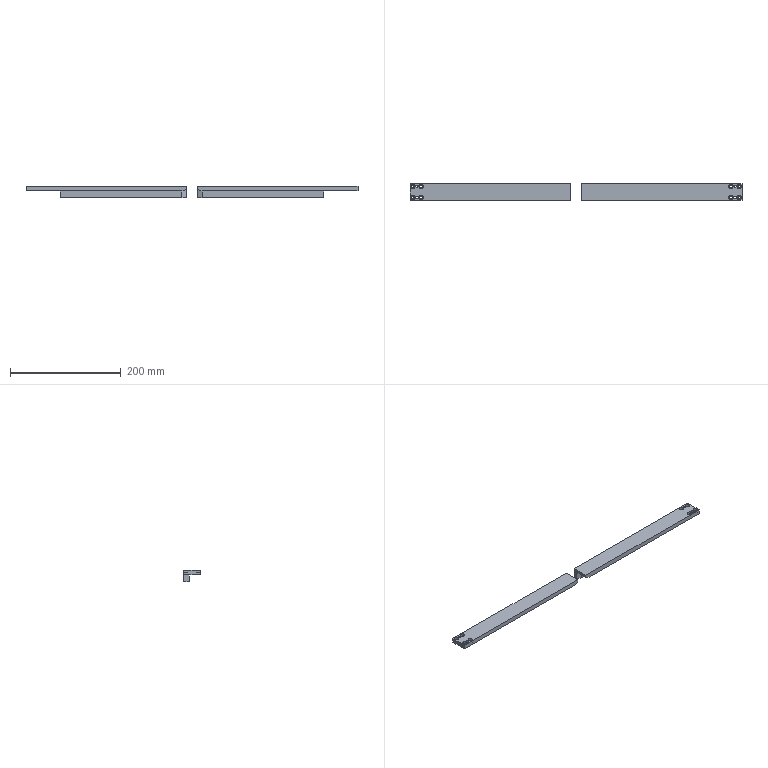NC program | NX | posted with a generic post | part box 600 x 30 x 20 mm
Whole program:
N10 G17 G21 G94 G90
(FLOOR_WALL_COPY_1 , TOOL : D50)
N12 T01 M6
N14 G54
N16 G17 G0 G90 X173. Y0. S6500 M3
N18 G43 Z30. H1
N20 Z7.
N22 G94 G1 Z4. F1250.
N24 X170.
N26 X-170.
N28 X-173.
N30 Z7.
N32 G0 Z30.
N34 X173.
N36 Z6.
N38 G1 Z3.
N40 X170.
N42 X-170.
N44 X-173.
N46 Z6.
N48 G0 Z30.
N50 X173.
N52 Z5.
N54 G1 Z2.
N56 X170.
N58 X-170.
N60 X-173.
N62 Z5.
N64 G0 Z30.
N66 X173.
N68 Z4.
N70 G1 Z1.
N72 X170.
N74 X-170.
N76 X-173.
N78 Z4.
N80 G0 Z30.
N82 X173.
N84 Z3.
N86 G1 Z0.
N88 X170.
N90 X-170.
N92 X-173.
N94 Z3.
N96 G0 Z30.
N98 M5
(FLOOR_WALL_1_1 , TOOL : D10)
N100 T03 M6
N102 G54
N104 G17 G0 G90 X-148.459 Y-23.147 S7000 M3
N106 G43 Z30. H3
N108 Z-8.85
N110 G94 G1 Z-11.85 F1000.
N112 X-149.446 Y-20.147
N114 G2 X-150.147 Y-17.873 R64. F3000.
N116 G1 Y-13.829
N118 G3 X-148.392 Y-20.147 R63.
N120 G1 X-147.337
N122 G2 X-150.147 Y-8.032 R62.
N124 G1 X-150.528 Y-5.056
N126 X-153.147
N128 Z-8.85
N130 G0 Z30.
N132 X-149.65 Y23.147
N134 Z-8.85
N136 G1 Z-11.85 F1000.
N138 Y20.147
N140 Y-0.15 F3000.
N142 G3 X-146.279 Y-20.147 R61.
N144 G1 X-145.22
N146 G2 X-148.65 Y-0.15 R60.
N148 G1 Y20.147
N150 X-147.65
N152 Y-0.15
N154 G3 X-144.158 Y-20.147 R59.
N156 G1 X-143.094
N158 G2 X-146.65 Y-0.15 R58.
N160 G1 Y20.147
N162 X-145.65
N164 Y-0.15
N166 G3 X-142.027 Y-20.147 R57.
N168 G1 X-140.958
N170 G2 X-144.65 Y-0.15 R56.
N172 G1 Y20.147
N174 X-143.65
N176 Y-0.15
N178 G3 X-139.886 Y-20.147 R55.
N180 G1 X-138.811
N182 G2 X-142.65 Y-0.15 R54.
N184 G1 Y20.147
N186 X-141.65
N188 Y-0.15
N190 G3 X-137.733 Y-20.147 R53.
N192 G1 X-136.651
N194 G2 X-140.65 Y-0.15 R52.
N196 G1 Y20.147
N198 X-139.65
N200 Y-0.15
N202 G3 X-135.566 Y-20.147 R51.
N204 G1 X-134.477
N206 G2 X-138.65 Y-0.15 R50.
N208 G1 Y20.147
N210 X-137.65
N212 Y-0.15
N214 G3 X-133.384 Y-20.147 R49.
N216 G1 X-132.286
N218 G2 X-136.65 Y-0.15 R48.
N220 G1 Y20.147
N222 X-135.65
N224 Y-0.15
N226 G3 X-131.184 Y-20.147 R47.
N228 G1 X-130.076
N230 G2 X-134.65 Y-0.15 R46.
N232 G1 Y20.147
N234 X-133.65
N236 Y-0.15
N238 G3 X-128.963 Y-20.147 R45.
N240 G1 X-127.843
N242 G2 X-132.65 Y-0.15 R44.
N244 G1 Y20.147
N246 X-131.65
N248 Y-0.15
N250 G3 X-126.717 Y-20.147 R43.
N252 G1 X-125.584
N254 G2 X-130.65 Y-0.15 R42.
N256 G1 Y20.147
N258 X-129.65
N260 Y-0.15
N262 G3 X-124.443 Y-20.147 R41.
N264 G1 X-123.293
N266 G2 X-128.65 Y-0.15 R40.
N268 G1 Y20.147
N270 X-127.65
N272 Y-0.15
N274 G3 X-122.133 Y-20.147 R39.
N276 G1 X-120.963
N278 G2 X-126.65 Y-0.15 R38.
N280 G1 Y20.147
N282 X-125.65
N284 Y-0.15
N286 G3 X-119.781 Y-20.147 R37.
N288 G1 X-118.585
N290 G2 X-124.65 Y-0.15 R36.
N292 G1 Y20.147
N294 X-123.65
N296 Y-0.15
N298 G3 X-117.375 Y-20.147 R35.
N300 G1 X-116.148
N302 G2 X-122.65 Y-0.15 R34.
N304 G1 Y20.147
N306 X-121.65
N308 Y-0.15
N310 G3 X-114.901 Y-20.147 R33.
N312 G1 X-113.632
N314 G2 X-120.65 Y-0.15 R32.
N316 G1 Y20.147
N318 X-119.65
N320 Y-0.15
N322 G3 X-112.338 Y-20.147 R31.
N324 G1 X-111.013
N326 G2 X-118.65 Y-0.15 R30.
N328 G1 Y20.147
N330 X-117.65
N332 Y-0.15
N334 G3 X-109.653 Y-20.147 R29.
N336 G1 X-108.249
N338 G2 X-116.65 Y-0.15 R28.
N340 G1 Y20.147
N342 X-115.65
N344 Y-0.15
N346 G3 X-106.792 Y-20.147 R27.
N348 G1 X-105.267
N350 G2 X-114.65 Y-0.15 R26.
N352 G1 Y20.147
N354 X-113.65
N356 Y-0.15
N358 G3 X-103.654 Y-20.147 R25.
N360 G1 X-101.921
N362 G2 X-112.65 Y-0.15 R24.
N364 G1 Y20.147
N366 X-111.65
N368 Y-0.15
N370 G3 X-100.013 Y-20.147 R23.
N372 G1 X-97.822
N374 G2 X-110.65 Y-0.15 R22.
N376 G1 Y20.147
N378 X-109.65
N380 Y-0.15
N382 G3 X-95.062 Y-20.147 R21.
N384 G1 X-88.996
N386 G2 X-108.65 Y-0.15 R20.
N388 G1 Y20.147
N390 Y23.147
N392 Z-8.85
N394 G0 Z30.
N396 X141.729 Y-23.147
N398 Z-8.85
N400 G1 Z-11.85 F1000.
N402 X149.972 Y-20.147
N404 X150.147 Y-20.083 F3000.
N406 Y-19.019
N408 X147.048 Y-20.147
N410 X144.078
N412 G3 X144.848 Y-19.884 R21.
N414 G1 X150.147 Y-17.955
N416 Y-16.891
N418 X144.506 Y-18.944
N420 G2 X138.012 Y-20.147 R20.
N422 G1 X135.012 Y-20.199
N424 Y-23.147
N426 Z-8.85
N428 G0 Z30.
N430 X-107.65 Y23.147
N432 Z-8.85
N434 G1 Z-11.85 F1000.
N436 Y20.147
N438 Y-0.15 F3000.
N440 G3 X-88.65 Y-19.15 R19.
N442 G1 X137.666
N444 G3 X144.164 Y-18.004 R19.
N446 G1 X150.147 Y-15.827
N448 Y-15.
N450 Y-14.762
N452 X143.822 Y-17.064
N454 G2 X137.666 Y-18.15 R18.
N456 G1 X-88.65
N458 G2 X-106.65 Y-0.15 R18.
N460 G1 Y20.147
N462 X-105.65
N464 Y-0.15
N466 G3 X-88.65 Y-17.15 R17.
N468 G1 X137.666
N470 G3 X143.48 Y-16.125 R17.
N472 G1 X150.147 Y-13.698
N474 Y-12.634
N476 X143.138 Y-15.185
N478 G2 X137.666 Y-16.15 R16.
N480 G1 X-88.65
N482 G2 X-104.65 Y-0.15 R16.
N484 G1 Y20.147
N486 X-103.65
N488 Y-0.15
N490 G3 X-88.65 Y-15.15 R15.
N492 G1 X137.666
N494 G3 X142.796 Y-14.245 R15.
N496 G1 X150.147 Y-11.57
N498 Y-10.506
N500 X142.454 Y-13.306
N502 G2 X137.666 Y-14.15 R14.
N504 G1 X-88.65
N506 G2 X-102.65 Y-0.15 R14.
N508 G1 Y20.147
N510 X-101.65
N512 Y-0.15
N514 G3 X-88.65 Y-13.15 R13.
N516 G1 X137.666
N518 G3 X142.112 Y-12.366 R13.
N520 G1 X150.147 Y-9.441
N522 Y-8.377
N524 X141.77 Y-11.426
N526 G2 X137.666 Y-12.15 R12.
N528 G1 X-88.65
N530 G2 X-100.65 Y-0.15 R12.
N532 G1 Y20.147
N534 X-99.65
N536 Y-0.15
N538 G3 X-88.65 Y-11.15 R11.
N540 G1 X137.666
N542 G3 X141.428 Y-10.487 R11.
N544 G1 X150.147 Y-7.313
N546 Y-6.249
N548 X141.086 Y-9.547
N550 G2 X137.666 Y-10.15 R10.
N552 G1 X-88.65
N554 G2 X-98.65 Y-0.15 R10.
N556 G1 Y20.147
N558 X-97.65
N560 Y-0.15
N562 G3 X-88.65 Y-9.15 R9.
N564 G1 X137.666
N566 G3 X140.744 Y-8.607 R9.
N568 G1 X150.147 Y-5.185
N570 Y-4.121
N572 X140.402 Y-7.668
N574 G2 X137.666 Y-8.15 R8.
N576 G1 X-88.65
N578 G2 X-96.65 Y-0.15 R8.
N580 G1 Y20.147
N582 X-95.65
N584 Y-0.15
N586 G3 X-88.65 Y-7.15 R7.
N588 G1 X137.666
N590 G3 X140.06 Y-6.728 R7.
N592 G1 X150.147 Y-3.056
N594 Y-1.992
N596 X139.718 Y-5.788
N598 G2 X137.666 Y-6.15 R6.
N600 G1 X-88.65
N602 G2 X-94.65 Y-0.15 R6.
N604 G1 Y20.147
N606 X-93.65
N608 Y-0.15
N610 G3 X-88.65 Y-5.15 R5.
N612 G1 X137.666
N614 G3 X139.376 Y-4.848 R5.
N616 G1 X150.147 Y-0.928
N618 Y0.136
N620 X139.034 Y-3.909
N622 G2 X137.666 Y-4.15 R4.
N624 G1 X-88.65
N626 G2 X-92.65 Y-0.15 R4.
N628 G1 Y20.147
N630 X-91.65
N632 Y-0.15
N634 G3 X-88.65 Y-3.15 R3.
N636 G1 X137.666
N638 G3 X138.692 Y-2.969 R3.
N640 G1 X150.147 Y1.2
N642 Y2.264
N644 X138.35 Y-2.029
N646 G2 X137.666 Y-2.15 R2.
N648 G1 X-88.65
N650 G2 X-90.65 Y-0.15 R2.
N652 G1 Y20.147
N654 X-89.65
N656 Y-0.15
N658 G3 X-88.65 Y-1.15 R1.
N660 G1 X137.666
N662 G3 X138.008 Y-1.09 R1.
N664 G1 X150.147 Y3.329
N666 Y4.393
N668 X137.666 Y-0.15
N670 X-88.65
N672 Y20.147
N674 Y23.15
N676 Z-8.85
N678 G0 Z30.
N680 M5
(FLOOR_WALL_1_COPY_1_1 , TOOL : D10JING)
N682 T04 M6
N684 G54
N686 G17 G0 G90 X151.139 Y-20.974 S7000 M3
N688 G43 Z30. H4
N690 Z-10.5
N692 G94 G1 Z-12. F1000.
N694 X150.865 Y-20.499
N696 G3 X149.999 Y-19.999 R1.
N698 G1 X-149.999
N700 Y-15.571
N702 X149.999
N704 Y-11.142
N706 X-149.999
N708 Y-6.714
N710 X149.999
N712 Y-2.286
N714 X-149.999
N716 Y2.142
N718 X-89.
N720 Y6.571
N722 X-149.999
N724 Y10.999
N726 X-89.
N728 Y15.427
N730 X-149.999
N732 G3 X-150.865 Y14.927 R1.
N734 G1 X-151.499 Y13.829
N736 Z-10.5
N738 G0 Z-8.9
N740 G1 X-89. Y2.142 F6000.
N742 G0 Z-10.5
N744 G1 Z-12. F1000.
N746 Y0.
N748 G3 X-88.5 Y-0.5 R0.5
N750 G1 X137.639
N752 X137.728 Y-0.502
N754 X137.81 Y-0.47
N756 X144.987 Y2.142
N758 X149.999
N760 G2 X150.865 Y1.642 R1.
N762 G1 X151.499 Y0.544
N764 Z-10.5
N766 G0 Z-8.9
N768 G1 X151.5 Y3.892 F6000.
N770 G0 Z-10.5
N772 G1 Z-12. F1000.
N774 X150.984 Y4.325
N776 G3 X149.999 Y4.499 R1.
N778 G1 X137.639 Y0.
N780 X-88.5
N782 Y19.999
N784 G3 X-89. Y20.865 R1.
N786 G1 X-90.098 Y21.499
N788 Z-10.5
N790 G0 Z30.
N792 M5
(ZLEVEL_PROFILE_COPY_COPY_1_COPY_COPY_COPY_1_COPY_COPY_1 , TOOL : D6R0.5)
N794 T20 M6
N796 G54
N798 G17 G0 G90 X139.958 Y-16.121 S7000 M3
N800 G43 Z30. H20
N802 Z-12.034
N804 G94 G1 X139.738 Y-15.994 F1000.
N806 G2 X139.439 Y-15.474 R0.6
N808 G1 X139.44 Y-15. F3000.
N810 Y2.784
N812 X139.534 Y2.818 Z-12.068
N814 Y-15.
N816 X139.533 Y-15.474
N818 X139.581 Y-15.475 Z-12.086
N820 X139.627 Z-12.103
N822 X139.628 Y-15.
N824 Y2.852
N826 X139.722 Y2.886 Z-12.137
N828 Y-15.
N830 X139.721 Y-15.476
N832 X139.769 Z-12.154
N834 X139.815 Z-12.171
N836 X139.816 Y-15.
N838 Y2.92
N840 X139.91 Y2.955 Z-12.205
N842 Y-15.
N844 X139.909 Y-15.477
N846 X139.957 Z-12.222
N848 X140.003 Z-12.239
N850 X140.004 Y-15.
N852 Y2.989
N854 X140.097 Y3.023 Z-12.274
N856 Y-15.
N858 Y-15.478
N860 X140.144 Z-12.291
N862 X140.191 Y-15.479 Z-12.308
N864 Y-15.
N866 Y3.057
N868 X140.285 Y3.092 Z-12.342
N870 Y-15.
N872 Y-15.479
N874 X140.332 Y-15.48 Z-12.359
N876 X140.379 Z-12.376
N878 Y-15.
N880 Y3.126
N882 X140.473 Y3.16 Z-12.41
N884 Y-15.
N886 Y-15.48
N888 X140.52 Y-15.481 Z-12.428
N890 X140.567 Z-12.445
N892 Y-15.
N894 Y3.194
N896 X140.661 Y3.228 Z-12.479
N898 Y-15.
N900 Y-15.482
N902 X140.708 Z-12.496
N904 X140.755 Z-12.513
N906 Y-15.
N908 Y3.263
N910 X140.849 Y3.297 Z-12.547
N912 Y-15.
N914 Y-15.483
N916 X140.896 Z-12.564
N918 X140.943 Y-15.484 Z-12.581
N920 Y-15.
N922 Y3.331
N924 X141.037 Y3.365 Z-12.616
N926 Y-15.
N928 Y-15.484
N930 X141.084 Z-12.633
N932 X141.131 Y-15.485 Z-12.65
N934 Y-15.
N936 Y3.399
N938 X141.225 Y3.434 Z-12.684
N940 Y-15.
N942 Y-15.485
N944 X141.272 Z-12.701
N946 X141.319 Y-15.486 Z-12.718
N948 Y-15.
N950 Y3.468
N952 X141.413 Y3.502 Z-12.752
N954 Y-15.
N956 Y-15.486
N958 X141.46 Z-12.77
N960 X141.506 Z-12.787
N962 X141.507 Y-15.
N964 Y3.536
N966 X141.601 Y3.57 Z-12.821
N968 Y-15.
N970 X141.6 Y-15.487
N972 X141.648 Z-12.838
N974 X141.694 Z-12.855
N976 X141.695 Y-15.
N978 Y3.605
N980 X141.789 Y3.639 Z-12.889
N982 Y-15.
N984 X141.788 Y-15.487
N986 X141.836 Y-15.488 Z-12.906
N988 X141.882 Z-12.923
N990 X141.883 Y-15.
N992 Y3.673
N994 X141.977 Y3.707 Z-12.958
N996 Y-15.
N998 X141.976 Y-15.488
N1000 X142.024 Z-12.975
N1002 X142.07 Y-15.489 Z-12.992
N1004 X142.071 Y-15.
N1006 Y3.741
N1008 X142.165 Y3.776 Z-13.026
N1010 Y-15.
N1012 X142.164 Y-15.489
N1014 X142.212 Z-13.043
N1016 X142.258 Z-13.06
N1018 X142.259 Y-15.
N1020 Y3.81
N1022 X142.353 Y3.844 Z-13.094
N1024 Y-15.
N1026 X142.352 Y-15.49
N1028 X142.4 Z-13.112
N1030 X142.446 Z-13.129
N1032 X142.447 Y-15.
N1034 Y3.878
N1036 X142.541 Y3.912 Z-13.163
N1038 Y-15.
N1040 X142.54 Y-15.491
N1042 X142.588 Z-13.18
N1044 X142.634 Z-13.197
N1046 X142.635 Y-15.
N1048 Y3.947
N1050 X142.729 Y3.981 Z-13.231
N1052 Y-15.
N1054 X142.728 Y-15.491
N1056 X142.776 Z-13.248
N1058 X142.822 Z-13.265
N1060 X142.823 Y-15.
N1062 Y4.015
N1064 X142.917 Y4.049 Z-13.3
N1066 Y-15.
N1068 X142.916 Y-15.491
N1070 X142.964 Z-13.317
N1072 X143.01 Z-13.334
N1074 X143.011 Y-15.
N1076 Y4.083
N1078 X143.105 Y4.118 Z-13.368
N1080 Y-15.
N1082 X143.104 Y-15.491
N1084 X143.151 Z-13.385
N1086 X143.198 Z-13.402
N1088 Y-15.
N1090 Y4.152
N1092 X143.292 Y4.186 Z-13.436
N1094 Y-15.
N1096 Y-15.491
N1098 X143.339 Z-13.454
N1100 X143.386 Z-13.471
N1102 Y-15.
N1104 Y4.22
N1106 X143.48 Y4.254 Z-13.505
N1108 Y-15.
N1110 Y-15.491
N1112 X143.527 Z-13.522
N1114 X143.574 Z-13.539
N1116 Y-15.
N1118 Y4.289
N1120 X143.668 Y4.323 Z-13.573
N1122 Y-15.
N1124 Y-15.491
N1126 X143.715 Z-13.59
N1128 X143.762 Z-13.607
N1130 Y-15.
N1132 Y4.357
N1134 X143.856 Y4.391 Z-13.642
N1136 Y-15.
N1138 Y-15.491
N1140 X143.903 Z-13.659
N1142 X143.95 Z-13.676
N1144 Y-15.
N1146 Y4.425
N1148 X144.044 Y4.46 Z-13.71
N1150 Y-15.
N1152 Y-15.491
N1154 X144.091 Z-13.727
N1156 X144.138 Z-13.744
N1158 Y-15.
N1160 Y4.494
N1162 X144.232 Y4.528 Z-13.779
N1164 Y-15.
N1166 Y-15.491
N1168 X144.279 Z-13.796
N1170 X144.326 Z-13.813
N1172 Y-15.
N1174 Y4.562
N1176 X144.42 Y4.596 Z-13.847
N1178 Y-15.
N1180 Y-15.491
N1182 X144.467 Z-13.864
N1184 X144.514 Z-13.881
N1186 Y-15.
N1188 Y4.631
N1190 X144.608 Y4.665 Z-13.915
N1192 Y-15.
N1194 Y-15.49
N1196 X144.655 Z-13.932
N1198 X144.701 Z-13.95
N1200 X144.702 Y-15.
N1202 Y4.699
N1204 X144.796 Y4.733 Z-13.984
N1206 Y-15.
N1208 X144.795 Y-15.49
N1210 X144.843 Y-15.489 Z-14.001
N1212 X144.889 Z-14.018
N1214 X144.89 Y-15.
N1216 Y4.767
N1218 X144.984 Y4.802 Z-14.052
N1220 Y-15.
N1222 X144.983 Y-15.489
N1224 X145.031 Z-14.069
N1226 X145.077 Y-15.488 Z-14.086
N1228 X145.078 Y-15.
N1230 Y4.836
N1232 X145.172 Y4.87 Z-14.121
N1234 Y-15.
N1236 X145.171 Y-15.488
N1238 X145.219 Z-14.138
N1240 X145.265 Z-14.155
N1242 X145.266 Y-15.
N1244 Y4.904
N1246 X145.36 Y4.938 Z-14.189
N1248 Y-15.
N1250 X145.359 Y-15.487
N1252 X145.407 Z-14.206
N1254 X145.453 Z-14.223
N1256 X145.454 Y-15.
N1258 Y4.973
N1260 X145.548 Y5.007 Z-14.257
N1262 Y-15.
N1264 X145.547 Y-15.487
N1266 X145.595 Y-15.486 Z-14.274
N1268 X145.641 Z-14.292
N1270 X145.642 Y-15.
N1272 Y5.041
N1274 X145.736 Y5.075 Z-14.326
N1276 Y-15.
N1278 X145.735 Y-15.486
N1280 X145.783 Z-14.343
N1282 X145.829 Y-15.485 Z-14.36
N1284 X145.83 Y-15.
N1286 Y5.109
N1288 X145.924 Y5.144 Z-14.394
N1290 Y-15.
N1292 X145.923 Y-15.485
N1294 X145.971 Z-14.411
N1296 X146.017 Z-14.428
N1298 X146.018 Y-15.
N1300 Y5.178
N1302 X146.112 Y5.214 Z-14.463
N1304 Y-15.
N1306 X146.111 Y-15.484
N1308 X146.159 Z-14.48
N1310 X146.205 Y-15.483 Z-14.497
N1312 Y-15.
N1314 Y5.253
N1316 X146.299 Y5.296 Z-14.531
N1318 Y-15.
N1320 Y-15.483
N1322 X146.346 Y-15.482 Z-14.548
N1324 X146.393 Z-14.565
N1326 Y-15.
N1328 Y5.343
N1330 X146.487 Y5.395 Z-14.599
N1332 Y-15.
N1334 Y-15.482
N1336 X146.534 Y-15.481 Z-14.616
N1338 X146.581 Z-14.634
N1340 Y-15.
N1342 Y5.451
N1344 X146.675 Y5.511 Z-14.668
N1346 Y-15.
N1348 Y-15.48
N1350 X146.722 Z-14.685
N1352 X146.769 Z-14.702
N1354 Y-15.
N1356 Y5.577
N1358 X146.863 Y5.649 Z-14.736
N1360 Y-15.
N1362 Y-15.479
N1364 X146.91 Z-14.753
N1366 X146.957 Y-15.478 Z-14.77
N1368 Y-15.
N1370 Y5.726
N1372 X147.051 Y5.811 Z-14.805
N1374 Y-15.
N1376 Y-15.478
N1378 X147.098 Y-15.477 Z-14.822
N1380 X147.144 Z-14.839
N1382 X147.145 Y-15.
N1384 Y5.903
N1386 X147.239 Y6.003 Z-14.873
N1388 Y-15.
N1390 X147.238 Y-15.476
N1392 X147.286 Z-14.89
N1394 X147.332 Z-14.907
N1396 X147.333 Y-15.
N1398 Y6.114
N1400 X147.427 Y6.237 Z-14.941
N1402 Y-15.
N1404 X147.426 Y-15.475
N1406 X147.474 Z-14.958
N1408 X147.52 Z-14.976
N1410 X147.521 Y-15.
N1412 Y6.374
N1414 X147.57 Y6.452 Z-14.993
N1416 X147.615 Y6.53 Z-15.01
N1418 Y-15.
N1420 X147.614 Y-15.474
N1422 X147.662 Z-15.027
N1424 X147.708 Y-15.473 Z-15.044
N1426 X147.709 Y6.572
N1428 X147.798 Y6.918
N1430 X147.839 Y7.032 Z-15.055
N1432 X147.876 Y7.147 Z-15.067
N1434 X147.908 Y7.263 Z-15.078
N1436 X147.803 Y6.918
N1438 X147.802 Y-15.473
N1440 X147.85 Y-15.472 Z-15.095
N1442 X147.896 Z-15.112
N1444 X147.897 Y6.918
N1446 X147.908 Y7.263
N1448 X147.941 Y7.41 Z-15.119
N1450 X147.967 Y7.557 Z-15.126
N1452 X147.985 Y7.705 Z-15.133
N1454 X147.996 Y7.852 Z-15.14
N1456 X148. Y8. Z-15.147
N1458 X147.991 Y7.762
N1460 X147.99 Y-15.465
N1462 X148.038 Y-15.365 Z-15.164
N1464 X148.084 Y-15.264 Z-15.181
N1466 X148.085 Y8.646
N1468 G2 X148.385 Y9.165 R0.6
N1470 G1 X148.61 Y9.295
N1472 G0 Z30.
N1474 M5
(ZLEVEL_PROFILE_COPY_1_COPY_COPY_COPY_COPY_2_COPY_COPY_1 , TOOL : D6A45)
N1476 T02 M6
N1478 G54
N1480 G17 G0 G90 X-84.421 Y16.953 S7000 M3
N1482 G43 Z30. H2
N1484 Z-1.
N1486 G94 G1 X-84.02 Y16.259 F1000.
N1488 G3 X-83.501 Y15.959 R0.6
N1490 G1 X145.001
N1492 G2 X145.959 Y15.001 R0.966
N1494 G1 Y7.999
N1496 G2 X145.329 Y7.1 R0.957
N1498 G1 X137.085 Y4.099
N1500 G2 X136.758 Y4.041 R0.954
N1502 G1 X-83.501
N1504 G2 X-84.459 Y4.999 R0.958
N1506 G1 Y15.001
N1508 G2 X-83.501 Y15.959 R0.958
N1510 G3 X-82.981 Y16.259 R0.6
N1512 G1 X-82.461 Y17.159
N1514 G0 Z30.
(ZLEVEL_PROFILE_COPY_1_COPY_COPY_COPY_COPY_2_COPY_COPY_COPY_1 , TOOL : D6A45)
N1516 X-124.958 Y10.081
N1518 Z-13.
N1520 G1 X-124.48 Y10.991
N1522 G3 X-125. Y11.291 R0.6
N1524 X-126.291 Y10. R1.291
N1526 X-125. Y11.291 R-1.291
N1528 X-125.52 Y10.991 R0.6
N1530 G1 X-125.042 Y10.081
N1532 G0 Z30.
N1534 X-139.958
N1536 Z-13.
N1538 G1 X-139.48 Y10.991
N1540 G3 X-140. Y11.291 R0.6
N1542 X-141.291 Y10. R1.291
N1544 X-140. Y11.291 R-1.291
N1546 X-140.52 Y10.991 R0.6
N1548 G1 X-140.042 Y10.081
N1550 G0 Z30.
N1552 Y-10.081
N1554 Z-13.
N1556 G1 X-140.52 Y-10.991
N1558 G3 X-140. Y-11.291 R0.6
N1560 X-138.709 Y-10. R1.291
N1562 X-140. Y-11.291 R-1.291
N1564 X-139.48 Y-10.991 R0.6
N1566 G1 X-139.958 Y-10.081
N1568 G0 Z30.
N1570 X-125.042
N1572 Z-13.
N1574 G1 X-125.52 Y-10.991
N1576 G3 X-125. Y-11.291 R0.6
N1578 X-123.709 Y-10. R1.291
N1580 X-125. Y-11.291 R-1.291
N1582 X-124.48 Y-10.991 R0.6
N1584 G1 X-124.958 Y-10.081
N1586 G0 Z30.
N1588 X-131.459 Y-10.5
N1590 Z-12.
N1592 G1 Z-13.
N1594 Y-9.5
N1596 G3 X-132.5 Y-8.459 R1.041
N1598 X-133.541 Y-9.5 R1.041
N1600 G1 Y-10.5
N1602 G3 X-132.5 Y-11.541 R1.041
N1604 X-131.459 Y-10.5 R1.041
N1606 X-131.759 Y-9.98 R0.6
N1608 G0 Z30.
N1610 X-132.5 Y11.041
N1612 Z-12.
N1614 G1 Z-13.
N1616 G3 X-133.541 Y10. R1.041
N1618 X-132.5 Y11.041 R-1.041
N1620 X-133.02 Y10.741 R0.6
N1622 G0 Z30.
N1624 X137.681 Y-16.957
N1626 Z-13.
N1628 G1 X137.278 Y-16.259
N1630 G3 X136.758 Y-15.959 R0.6
N1632 G1 X-145.001
N1634 G2 X-145.959 Y-15.001 R0.958
N1636 G1 Y15.001
N1638 G2 X-145.001 Y15.959 R0.958
N1640 G1 X-86.665
N1642 G3 X-86.405 Y16.109 R0.3
N1644 G1 X-87.023 Y17.159
N1646 G0 Z30.
N1648 M5
N1650 M2